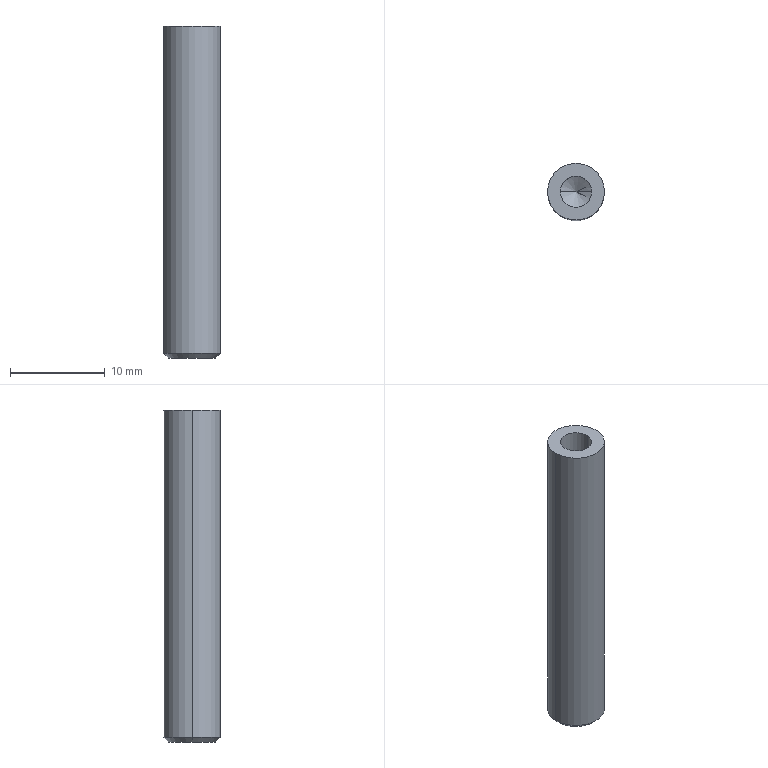Part | SolidWorks | features Chamfer 1, Extrusion 1, HoleWzd 1 | 1 solid | 10 faces | box 6 x 6 x 35 mm | volume 898.165 mm3 | cone 4 | cylinder 4 | plane 2 | commonest cylinder face diameters 3.3 x2 6 x2
STEP:
#1=CARTESIAN_POINT('',(-2.5,0.,-17.5));
#2=VERTEX_POINT('',#1);
#3=CARTESIAN_POINT('',(2.5,0.,-17.5));
#4=VERTEX_POINT('',#3);
#5=CARTESIAN_POINT('',(0.,0.,-17.5));
#6=DIRECTION('',(0.,0.,-1.));
#7=DIRECTION('',(1.,0.,0.));
#8=AXIS2_PLACEMENT_3D('',#5,#6,#7);
#9=CIRCLE('',#8,2.5);
#10=EDGE_CURVE('',#2,#4,#9,.T.);
#11=ORIENTED_EDGE('',*,*,#10,.F.);
#12=CARTESIAN_POINT('',(-3.,0.,-17.));
#13=VERTEX_POINT('',#12);
#14=CARTESIAN_POINT('',(-3.,0.,-17.));
#15=DIRECTION('',(-0.7071,0.,0.7071));
#16=VECTOR('',#15,1000.);
#17=LINE('',#14,#16);
#18=EDGE_CURVE('',#2,#13,#17,.T.);
#19=ORIENTED_EDGE('',*,*,#18,.T.);
#20=CARTESIAN_POINT('',(3.,0.,-17.));
#21=VERTEX_POINT('',#20);
#22=CARTESIAN_POINT('',(0.,0.,-17.));
#23=DIRECTION('',(0.,0.,1.));
#24=DIRECTION('',(1.,0.,0.));
#25=AXIS2_PLACEMENT_3D('',#22,#23,#24);
#26=CIRCLE('',#25,3.);
#27=EDGE_CURVE('',#21,#13,#26,.T.);
#28=ORIENTED_EDGE('',*,*,#27,.F.);
#29=CARTESIAN_POINT('',(3.,0.,-17.));
#30=DIRECTION('',(0.7071,0.,0.7071));
#31=VECTOR('',#30,1000.);
#32=LINE('',#29,#31);
#33=EDGE_CURVE('',#4,#21,#32,.T.);
#34=ORIENTED_EDGE('',*,*,#33,.F.);
#35=EDGE_LOOP('',(#11,#19,#28,#34));
#36=FACE_OUTER_BOUND('',#35,.T.);
#37=CARTESIAN_POINT('',(0.,0.,-17.));
#38=DIRECTION('',(0.,0.,1.));
#39=DIRECTION('',(1.,0.,0.));
#40=AXIS2_PLACEMENT_3D('',#37,#38,#39);
#41=CONICAL_SURFACE('',#40,3.,0.7854);
#42=ADVANCED_FACE('',(#36),#41,.T.);
#43=CARTESIAN_POINT('',(-1.65,0.,7.4));
#44=VERTEX_POINT('',#43);
#45=CARTESIAN_POINT('',(1.65,0.,7.4));
#46=VERTEX_POINT('',#45);
#47=CARTESIAN_POINT('',(0.,0.,7.4));
#48=DIRECTION('',(0.,0.,1.));
#49=DIRECTION('',(1.,0.,0.));
#50=AXIS2_PLACEMENT_3D('',#47,#48,#49);
#51=CIRCLE('',#50,1.65);
#52=EDGE_CURVE('',#44,#46,#51,.T.);
#53=ORIENTED_EDGE('',*,*,#52,.F.);
#54=CARTESIAN_POINT('',(-1.65,0.,17.5));
#55=VERTEX_POINT('',#54);
#56=CARTESIAN_POINT('',(-1.65,0.,17.5));
#57=DIRECTION('',(0.,0.,1.));
#58=VECTOR('',#57,1000.);
#59=LINE('',#56,#58);
#60=EDGE_CURVE('',#44,#55,#59,.T.);
#61=ORIENTED_EDGE('',*,*,#60,.T.);
#62=CARTESIAN_POINT('',(1.65,0.,17.5));
#63=VERTEX_POINT('',#62);
#64=CARTESIAN_POINT('',(0.,0.,17.5));
#65=DIRECTION('',(0.,0.,1.));
#66=DIRECTION('',(1.,0.,0.));
#67=AXIS2_PLACEMENT_3D('',#64,#65,#66);
#68=CIRCLE('',#67,1.65);
#69=EDGE_CURVE('',#55,#63,#68,.T.);
#70=ORIENTED_EDGE('',*,*,#69,.T.);
#71=CARTESIAN_POINT('',(1.65,0.,17.5));
#72=DIRECTION('',(0.,0.,1.));
#73=VECTOR('',#72,1000.);
#74=LINE('',#71,#73);
#75=EDGE_CURVE('',#46,#63,#74,.T.);
#76=ORIENTED_EDGE('',*,*,#75,.F.);
#77=EDGE_LOOP('',(#53,#61,#70,#76));
#78=FACE_OUTER_BOUND('',#77,.T.);
#79=CARTESIAN_POINT('',(0.,0.,17.5));
#80=DIRECTION('',(0.,0.,1.));
#81=DIRECTION('',(1.,0.,0.));
#82=AXIS2_PLACEMENT_3D('',#79,#80,#81);
#83=CYLINDRICAL_SURFACE('',#82,1.65);
#84=ADVANCED_FACE('',(#78),#83,.F.);
#85=CARTESIAN_POINT('',(0.,0.,6.409));
#86=VERTEX_POINT('',#85);
#87=CARTESIAN_POINT('',(1.65,0.,7.4));
#88=DIRECTION('',(0.8572,0.,0.515));
#89=VECTOR('',#88,1000.);
#90=LINE('',#87,#89);
#91=EDGE_CURVE('',#86,#46,#90,.T.);
#92=ORIENTED_EDGE('',*,*,#91,.F.);
#93=CARTESIAN_POINT('',(-1.65,0.,7.4));
#94=DIRECTION('',(-0.8572,0.,0.515));
#95=VECTOR('',#94,1000.);
#96=LINE('',#93,#95);
#97=EDGE_CURVE('',#86,#44,#96,.T.);
#98=ORIENTED_EDGE('',*,*,#97,.T.);
#99=ORIENTED_EDGE('',*,*,#52,.T.);
#100=EDGE_LOOP('',(#92,#98,#99));
#101=FACE_OUTER_BOUND('',#100,.T.);
#102=CARTESIAN_POINT('',(0.,0.,7.4));
#103=DIRECTION('',(0.,0.,1.));
#104=DIRECTION('',(1.,0.,0.));
#105=AXIS2_PLACEMENT_3D('',#102,#103,#104);
#106=CONICAL_SURFACE('',#105,1.65,1.03);
#107=ADVANCED_FACE('',(#101),#106,.F.);
#108=CARTESIAN_POINT('',(3.,0.,17.5));
#109=VERTEX_POINT('',#108);
#110=CARTESIAN_POINT('',(-3.,0.,17.5));
#111=VERTEX_POINT('',#110);
#112=CARTESIAN_POINT('',(0.,0.,17.5));
#113=DIRECTION('',(0.,0.,1.));
#114=DIRECTION('',(1.,0.,0.));
#115=AXIS2_PLACEMENT_3D('',#112,#113,#114);
#116=CIRCLE('',#115,3.);
#117=EDGE_CURVE('',#109,#111,#116,.T.);
#118=ORIENTED_EDGE('',*,*,#117,.F.);
#119=CARTESIAN_POINT('',(3.,0.,17.5));
#120=DIRECTION('',(0.,0.,-1.));
#121=VECTOR('',#120,1000.);
#122=LINE('',#119,#121);
#123=EDGE_CURVE('',#109,#21,#122,.T.);
#124=ORIENTED_EDGE('',*,*,#123,.T.);
#125=ORIENTED_EDGE('',*,*,#27,.T.);
#126=CARTESIAN_POINT('',(-3.,0.,17.5));
#127=DIRECTION('',(0.,0.,-1.));
#128=VECTOR('',#127,1000.);
#129=LINE('',#126,#128);
#130=EDGE_CURVE('',#111,#13,#129,.T.);
#131=ORIENTED_EDGE('',*,*,#130,.F.);
#132=EDGE_LOOP('',(#118,#124,#125,#131));
#133=FACE_OUTER_BOUND('',#132,.T.);
#134=CARTESIAN_POINT('',(0.,0.,17.5));
#135=DIRECTION('',(0.,0.,-1.));
#136=DIRECTION('',(-1.,0.,0.));
#137=AXIS2_PLACEMENT_3D('',#134,#135,#136);
#138=CYLINDRICAL_SURFACE('',#137,3.);
#139=ADVANCED_FACE('',(#133),#138,.T.);
#140=ORIENTED_EDGE('',*,*,#123,.F.);
#141=CARTESIAN_POINT('',(0.,0.,17.5));
#142=DIRECTION('',(0.,0.,1.));
#143=DIRECTION('',(1.,0.,0.));
#144=AXIS2_PLACEMENT_3D('',#141,#142,#143);
#145=CIRCLE('',#144,3.);
#146=EDGE_CURVE('',#111,#109,#145,.T.);
#147=ORIENTED_EDGE('',*,*,#146,.F.);
#148=ORIENTED_EDGE('',*,*,#130,.T.);
#149=CARTESIAN_POINT('',(0.,0.,-17.));
#150=DIRECTION('',(0.,0.,1.));
#151=DIRECTION('',(1.,0.,0.));
#152=AXIS2_PLACEMENT_3D('',#149,#150,#151);
#153=CIRCLE('',#152,3.);
#154=EDGE_CURVE('',#13,#21,#153,.T.);
#155=ORIENTED_EDGE('',*,*,#154,.T.);
#156=EDGE_LOOP('',(#140,#147,#148,#155));
#157=FACE_OUTER_BOUND('',#156,.T.);
#158=CARTESIAN_POINT('',(0.,0.,17.5));
#159=DIRECTION('',(0.,0.,-1.));
#160=DIRECTION('',(-1.,0.,0.));
#161=AXIS2_PLACEMENT_3D('',#158,#159,#160);
#162=CYLINDRICAL_SURFACE('',#161,3.);
#163=ADVANCED_FACE('',(#157),#162,.T.);
#164=CARTESIAN_POINT('',(0.,0.,17.5));
#165=DIRECTION('',(0.,0.,1.));
#166=DIRECTION('',(1.,0.,0.));
#167=AXIS2_PLACEMENT_3D('',#164,#165,#166);
#168=CIRCLE('',#167,1.65);
#169=EDGE_CURVE('',#63,#55,#168,.T.);
#170=ORIENTED_EDGE('',*,*,#169,.F.);
#171=ORIENTED_EDGE('',*,*,#69,.F.);
#172=EDGE_LOOP('',(#170,#171));
#173=FACE_BOUND('',#172,.T.);
#174=ORIENTED_EDGE('',*,*,#146,.T.);
#175=ORIENTED_EDGE('',*,*,#117,.T.);
#176=EDGE_LOOP('',(#174,#175));
#177=FACE_OUTER_BOUND('',#176,.T.);
#178=CARTESIAN_POINT('',(0.,0.,17.5));
#179=DIRECTION('',(0.,0.,1.));
#180=DIRECTION('',(1.,0.,0.));
#181=AXIS2_PLACEMENT_3D('',#178,#179,#180);
#182=PLANE('',#181);
#183=ADVANCED_FACE('',(#173,#177),#182,.T.);
#184=CARTESIAN_POINT('',(0.,0.,-17.5));
#185=DIRECTION('',(0.,0.,-1.));
#186=DIRECTION('',(1.,0.,0.));
#187=AXIS2_PLACEMENT_3D('',#184,#185,#186);
#188=CIRCLE('',#187,2.5);
#189=EDGE_CURVE('',#4,#2,#188,.T.);
#190=ORIENTED_EDGE('',*,*,#189,.T.);
#191=ORIENTED_EDGE('',*,*,#10,.T.);
#192=EDGE_LOOP('',(#190,#191));
#193=FACE_OUTER_BOUND('',#192,.T.);
#194=CARTESIAN_POINT('',(0.,0.,-17.5));
#195=DIRECTION('',(0.,0.,1.));
#196=DIRECTION('',(1.,0.,0.));
#197=AXIS2_PLACEMENT_3D('',#194,#195,#196);
#198=PLANE('',#197);
#199=ADVANCED_FACE('',(#193),#198,.F.);
#200=ORIENTED_EDGE('',*,*,#97,.F.);
#201=ORIENTED_EDGE('',*,*,#91,.T.);
#202=CARTESIAN_POINT('',(0.,0.,7.4));
#203=DIRECTION('',(0.,0.,1.));
#204=DIRECTION('',(1.,0.,0.));
#205=AXIS2_PLACEMENT_3D('',#202,#203,#204);
#206=CIRCLE('',#205,1.65);
#207=EDGE_CURVE('',#46,#44,#206,.T.);
#208=ORIENTED_EDGE('',*,*,#207,.T.);
#209=EDGE_LOOP('',(#200,#201,#208));
#210=FACE_OUTER_BOUND('',#209,.T.);
#211=CARTESIAN_POINT('',(0.,0.,7.4));
#212=DIRECTION('',(0.,0.,1.));
#213=DIRECTION('',(1.,0.,0.));
#214=AXIS2_PLACEMENT_3D('',#211,#212,#213);
#215=CONICAL_SURFACE('',#214,1.65,1.03);
#216=ADVANCED_FACE('',(#210),#215,.F.);
#217=ORIENTED_EDGE('',*,*,#60,.F.);
#218=ORIENTED_EDGE('',*,*,#207,.F.);
#219=ORIENTED_EDGE('',*,*,#75,.T.);
#220=ORIENTED_EDGE('',*,*,#169,.T.);
#221=EDGE_LOOP('',(#217,#218,#219,#220));
#222=FACE_OUTER_BOUND('',#221,.T.);
#223=CARTESIAN_POINT('',(0.,0.,17.5));
#224=DIRECTION('',(0.,0.,1.));
#225=DIRECTION('',(1.,0.,0.));
#226=AXIS2_PLACEMENT_3D('',#223,#224,#225);
#227=CYLINDRICAL_SURFACE('',#226,1.65);
#228=ADVANCED_FACE('',(#222),#227,.F.);
#229=ORIENTED_EDGE('',*,*,#18,.F.);
#230=ORIENTED_EDGE('',*,*,#189,.F.);
#231=ORIENTED_EDGE('',*,*,#33,.T.);
#232=ORIENTED_EDGE('',*,*,#154,.F.);
#233=EDGE_LOOP('',(#229,#230,#231,#232));
#234=FACE_OUTER_BOUND('',#233,.T.);
#235=CARTESIAN_POINT('',(0.,0.,-17.));
#236=DIRECTION('',(0.,0.,1.));
#237=DIRECTION('',(1.,0.,0.));
#238=AXIS2_PLACEMENT_3D('',#235,#236,#237);
#239=CONICAL_SURFACE('',#238,3.,0.7854);
#240=ADVANCED_FACE('',(#234),#239,.T.);
#241=CLOSED_SHELL('',(#42,#84,#107,#139,#163,#183,#199,#216,#228,#240));
#242=MANIFOLD_SOLID_BREP('',#241);
#243=CARTESIAN_POINT('',(0.,0.,0.));
#244=DIRECTION('',(0.,0.,1.));
#245=DIRECTION('',(1.,0.,0.));
#246=AXIS2_PLACEMENT_3D('',#243,#244,#245);
#247=(LENGTH_UNIT()NAMED_UNIT(*)SI_UNIT(.MILLI.,.METRE.));
#248=UNCERTAINTY_MEASURE_WITH_UNIT(LENGTH_MEASURE(0.00001),#247,'','');
#249=(NAMED_UNIT(*)PLANE_ANGLE_UNIT()SI_UNIT($,.RADIAN.));
#250=(NAMED_UNIT(*)SI_UNIT($,.STERADIAN.)SOLID_ANGLE_UNIT());
#251=(GEOMETRIC_REPRESENTATION_CONTEXT(3)GLOBAL_UNCERTAINTY_ASSIGNED_CONTEXT((#248))GLOBAL_UNIT_ASSIGNED_CONTEXT((#247,#249,#250))REPRESENTATION_CONTEXT('',''));
#252=ADVANCED_BREP_SHAPE_REPRESENTATION('',(#242,#246),#251);